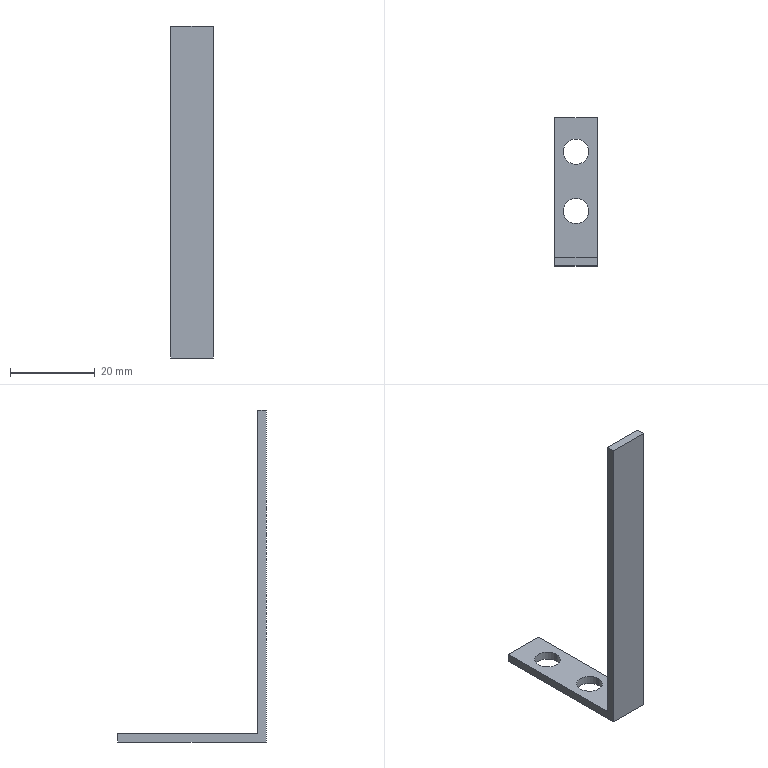Part | STEP file | 1_id1586_x_t | 1 solid | 12 faces | box 10 x 35 x 78.24 mm | volume 2112 mm3 | plane 8 | cylinder 4 | commonest cylinder face diameters 6 x4
STEP:
#1=CARTESIAN_POINT('',(0.,0.,0.));
#2=DIRECTION('',(0.,0.,1.));
#3=DIRECTION('',(1.,0.,0.));
#4=AXIS2_PLACEMENT_3D('',#1,#2,#3);
#5=CARTESIAN_POINT('',(897.895,192.425,-90.));
#6=VERTEX_POINT('',#5);
#7=CARTESIAN_POINT('',(897.895,192.425,-11.76));
#8=VERTEX_POINT('',#7);
#9=CARTESIAN_POINT('',(897.895,192.425,-90.));
#10=DIRECTION('',(0.,0.,1.));
#11=VECTOR('',#10,1.);
#12=LINE('',#9,#11);
#13=CARTESIAN_POINT('',(892.895,192.425,-50.88));
#14=DIRECTION('',(0.,1.,0.));
#15=DIRECTION('',(-1.,0.,0.));
#16=AXIS2_PLACEMENT_3D('',#13,#14,#15);
#17=PLANE('',#16);
#18=CARTESIAN_POINT('',(-5.,-39.12));
#19=DIRECTION('',(0.,1.));
#20=VECTOR('',#19,1.);
#21=LINE('',#18,#20);
#22=(GEOMETRIC_REPRESENTATION_CONTEXT(2)PARAMETRIC_REPRESENTATION_CONTEXT()REPRESENTATION_CONTEXT('',''));
#23=DEFINITIONAL_REPRESENTATION('',(#21),#22);
#24=PCURVE('',#17,#23);
#25=CARTESIAN_POINT('',(897.895,49.757,-105.374));
#26=DIRECTION('',(1.,0.,0.));
#27=DIRECTION('',(0.,-1.,0.));
#28=AXIS2_PLACEMENT_3D('',#25,#26,#27);
#29=PLANE('',#28);
#30=CARTESIAN_POINT('',(-142.668,-15.374));
#31=DIRECTION('',(0.,-1.));
#32=VECTOR('',#31,1.);
#33=LINE('',#30,#32);
#34=(GEOMETRIC_REPRESENTATION_CONTEXT(2)PARAMETRIC_REPRESENTATION_CONTEXT()REPRESENTATION_CONTEXT('',''));
#35=DEFINITIONAL_REPRESENTATION('',(#33),#34);
#36=PCURVE('',#29,#35);
#37=SURFACE_CURVE('',#12,(#24,#36),.PCURVE_S1.);
#38=EDGE_CURVE('',#6,#8,#37,.T.);
#39=ORIENTED_EDGE('',*,*,#38,.T.);
#40=CARTESIAN_POINT('',(887.895,192.425,-11.76));
#41=VERTEX_POINT('',#40);
#42=CARTESIAN_POINT('',(897.895,192.425,-11.76));
#43=DIRECTION('',(-1.,0.,0.));
#44=VECTOR('',#43,1.);
#45=LINE('',#42,#44);
#46=CARTESIAN_POINT('',(-5.,39.12));
#47=DIRECTION('',(1.,0.));
#48=VECTOR('',#47,1.);
#49=LINE('',#46,#48);
#50=(GEOMETRIC_REPRESENTATION_CONTEXT(2)PARAMETRIC_REPRESENTATION_CONTEXT()REPRESENTATION_CONTEXT('',''));
#51=DEFINITIONAL_REPRESENTATION('',(#49),#50);
#52=PCURVE('',#17,#51);
#53=CARTESIAN_POINT('',(902.895,192.425,-11.76));
#54=DIRECTION('',(0.,0.,-1.));
#55=DIRECTION('',(1.,0.,0.));
#56=AXIS2_PLACEMENT_3D('',#53,#54,#55);
#57=PLANE('',#56);
#58=CARTESIAN_POINT('',(-5.,0.));
#59=DIRECTION('',(-1.,0.));
#60=VECTOR('',#59,1.);
#61=LINE('',#58,#60);
#62=(GEOMETRIC_REPRESENTATION_CONTEXT(2)PARAMETRIC_REPRESENTATION_CONTEXT()REPRESENTATION_CONTEXT('',''));
#63=DEFINITIONAL_REPRESENTATION('',(#61),#62);
#64=PCURVE('',#57,#63);
#65=SURFACE_CURVE('',#45,(#52,#64),.PCURVE_S1.);
#66=EDGE_CURVE('',#8,#41,#65,.T.);
#67=ORIENTED_EDGE('',*,*,#66,.T.);
#68=CARTESIAN_POINT('',(887.895,192.425,-90.));
#69=VERTEX_POINT('',#68);
#70=CARTESIAN_POINT('',(887.895,192.425,-11.76));
#71=DIRECTION('',(0.,0.,-1.));
#72=VECTOR('',#71,1.);
#73=LINE('',#70,#72);
#74=CARTESIAN_POINT('',(5.,39.12));
#75=DIRECTION('',(0.,-1.));
#76=VECTOR('',#75,1.);
#77=LINE('',#74,#76);
#78=(GEOMETRIC_REPRESENTATION_CONTEXT(2)PARAMETRIC_REPRESENTATION_CONTEXT()REPRESENTATION_CONTEXT('',''));
#79=DEFINITIONAL_REPRESENTATION('',(#77),#78);
#80=PCURVE('',#17,#79);
#81=CARTESIAN_POINT('',(887.895,372.897,-105.638));
#82=DIRECTION('',(-1.,0.,0.));
#83=DIRECTION('',(0.,0.,-1.));
#84=AXIS2_PLACEMENT_3D('',#81,#82,#83);
#85=PLANE('',#84);
#86=CARTESIAN_POINT('',(-93.878,180.472));
#87=DIRECTION('',(1.,0.));
#88=VECTOR('',#87,1.);
#89=LINE('',#86,#88);
#90=(GEOMETRIC_REPRESENTATION_CONTEXT(2)PARAMETRIC_REPRESENTATION_CONTEXT()REPRESENTATION_CONTEXT('',''));
#91=DEFINITIONAL_REPRESENTATION('',(#89),#90);
#92=PCURVE('',#85,#91);
#93=SURFACE_CURVE('',#73,(#80,#92),.PCURVE_S1.);
#94=EDGE_CURVE('',#41,#69,#93,.T.);
#95=ORIENTED_EDGE('',*,*,#94,.T.);
#96=CARTESIAN_POINT('',(887.895,192.425,-90.));
#97=DIRECTION('',(1.,0.,0.));
#98=VECTOR('',#97,1.);
#99=LINE('',#96,#98);
#100=CARTESIAN_POINT('',(5.,-39.12));
#101=DIRECTION('',(-1.,0.));
#102=VECTOR('',#101,1.);
#103=LINE('',#100,#102);
#104=(GEOMETRIC_REPRESENTATION_CONTEXT(2)PARAMETRIC_REPRESENTATION_CONTEXT()REPRESENTATION_CONTEXT('',''));
#105=DEFINITIONAL_REPRESENTATION('',(#103),#104);
#106=PCURVE('',#17,#105);
#107=CARTESIAN_POINT('',(893.895,203.675,-90.));
#108=DIRECTION('',(0.,0.,-1.));
#109=DIRECTION('',(0.,1.,0.));
#110=AXIS2_PLACEMENT_3D('',#107,#108,#109);
#111=PLANE('',#110);
#112=CARTESIAN_POINT('',(-11.25,-6.));
#113=DIRECTION('',(0.,1.));
#114=VECTOR('',#113,1.);
#115=LINE('',#112,#114);
#116=(GEOMETRIC_REPRESENTATION_CONTEXT(2)PARAMETRIC_REPRESENTATION_CONTEXT()REPRESENTATION_CONTEXT('',''));
#117=DEFINITIONAL_REPRESENTATION('',(#115),#116);
#118=PCURVE('',#111,#117);
#119=SURFACE_CURVE('',#99,(#106,#118),.PCURVE_S1.);
#120=EDGE_CURVE('',#69,#6,#119,.T.);
#121=ORIENTED_EDGE('',*,*,#120,.T.);
#122=EDGE_LOOP('',(#39,#67,#95,#121));
#123=FACE_BOUND('',#122,.T.);
#124=ADVANCED_FACE('',(#123),#17,.F.);
#125=CARTESIAN_POINT('',(897.895,227.425,-90.));
#126=VERTEX_POINT('',#125);
#127=CARTESIAN_POINT('',(897.895,192.425,-90.));
#128=DIRECTION('',(0.,1.,0.));
#129=VECTOR('',#128,1.);
#130=LINE('',#127,#129);
#131=CARTESIAN_POINT('',(-11.25,4.));
#132=DIRECTION('',(1.,0.));
#133=VECTOR('',#132,1.);
#134=LINE('',#131,#133);
#135=(GEOMETRIC_REPRESENTATION_CONTEXT(2)PARAMETRIC_REPRESENTATION_CONTEXT()REPRESENTATION_CONTEXT('',''));
#136=DEFINITIONAL_REPRESENTATION('',(#134),#135);
#137=PCURVE('',#111,#136);
#138=CARTESIAN_POINT('',(-142.668,-15.374));
#139=DIRECTION('',(-1.,0.));
#140=VECTOR('',#139,1.);
#141=LINE('',#138,#140);
#142=(GEOMETRIC_REPRESENTATION_CONTEXT(2)PARAMETRIC_REPRESENTATION_CONTEXT()REPRESENTATION_CONTEXT('',''));
#143=DEFINITIONAL_REPRESENTATION('',(#141),#142);
#144=PCURVE('',#29,#143);
#145=SURFACE_CURVE('',#130,(#137,#144),.PCURVE_S1.);
#146=EDGE_CURVE('',#6,#126,#145,.T.);
#147=ORIENTED_EDGE('',*,*,#146,.F.);
#148=ORIENTED_EDGE('',*,*,#120,.F.);
#149=CARTESIAN_POINT('',(887.895,227.425,-90.));
#150=VERTEX_POINT('',#149);
#151=CARTESIAN_POINT('',(887.895,227.425,-90.));
#152=DIRECTION('',(0.,-1.,0.));
#153=VECTOR('',#152,1.);
#154=LINE('',#151,#153);
#155=CARTESIAN_POINT('',(23.75,-6.));
#156=DIRECTION('',(-1.,0.));
#157=VECTOR('',#156,1.);
#158=LINE('',#155,#157);
#159=(GEOMETRIC_REPRESENTATION_CONTEXT(2)PARAMETRIC_REPRESENTATION_CONTEXT()REPRESENTATION_CONTEXT('',''));
#160=DEFINITIONAL_REPRESENTATION('',(#158),#159);
#161=PCURVE('',#111,#160);
#162=CARTESIAN_POINT('',(-15.638,145.472));
#163=DIRECTION('',(0.,1.));
#164=VECTOR('',#163,1.);
#165=LINE('',#162,#164);
#166=(GEOMETRIC_REPRESENTATION_CONTEXT(2)PARAMETRIC_REPRESENTATION_CONTEXT()REPRESENTATION_CONTEXT('',''));
#167=DEFINITIONAL_REPRESENTATION('',(#165),#166);
#168=PCURVE('',#85,#167);
#169=SURFACE_CURVE('',#154,(#161,#168),.PCURVE_S1.);
#170=EDGE_CURVE('',#150,#69,#169,.T.);
#171=ORIENTED_EDGE('',*,*,#170,.F.);
#172=CARTESIAN_POINT('',(897.895,227.425,-90.));
#173=DIRECTION('',(-1.,0.,0.));
#174=VECTOR('',#173,1.);
#175=LINE('',#172,#174);
#176=CARTESIAN_POINT('',(23.75,4.));
#177=DIRECTION('',(0.,-1.));
#178=VECTOR('',#177,1.);
#179=LINE('',#176,#178);
#180=(GEOMETRIC_REPRESENTATION_CONTEXT(2)PARAMETRIC_REPRESENTATION_CONTEXT()REPRESENTATION_CONTEXT('',''));
#181=DEFINITIONAL_REPRESENTATION('',(#179),#180);
#182=PCURVE('',#111,#181);
#183=CARTESIAN_POINT('',(893.895,227.425,-90.));
#184=DIRECTION('',(0.,1.,0.));
#185=DIRECTION('',(-1.,0.,0.));
#186=AXIS2_PLACEMENT_3D('',#183,#184,#185);
#187=PLANE('',#186);
#188=CARTESIAN_POINT('',(-4.,0.));
#189=DIRECTION('',(1.,0.));
#190=VECTOR('',#189,1.);
#191=LINE('',#188,#190);
#192=(GEOMETRIC_REPRESENTATION_CONTEXT(2)PARAMETRIC_REPRESENTATION_CONTEXT()REPRESENTATION_CONTEXT('',''));
#193=DEFINITIONAL_REPRESENTATION('',(#191),#192);
#194=PCURVE('',#187,#193);
#195=SURFACE_CURVE('',#175,(#182,#194),.PCURVE_S1.);
#196=EDGE_CURVE('',#126,#150,#195,.T.);
#197=ORIENTED_EDGE('',*,*,#196,.F.);
#198=EDGE_LOOP('',(#147,#148,#171,#197));
#199=FACE_BOUND('',#198,.T.);
#200=CARTESIAN_POINT('',(895.895,219.425,-90.));
#201=VERTEX_POINT('',#200);
#202=CARTESIAN_POINT('',(889.895,219.425,-90.));
#203=VERTEX_POINT('',#202);
#204=CARTESIAN_POINT('',(892.895,219.425,-90.));
#205=DIRECTION('',(0.,0.,1.));
#206=DIRECTION('',(1.,0.,0.));
#207=AXIS2_PLACEMENT_3D('',#204,#205,#206);
#208=CIRCLE('',#207,3.);
#209=CARTESIAN_POINT('',(15.75,2.));
#210=CARTESIAN_POINT('',(20.946,2.));
#211=CARTESIAN_POINT('',(18.348,-2.5));
#212=CARTESIAN_POINT('',(15.75,-7.));
#213=CARTESIAN_POINT('',(13.152,-2.5));
#214=CARTESIAN_POINT('',(10.554,2.));
#215=CARTESIAN_POINT('',(15.75,2.));
#216=(BOUNDED_CURVE()B_SPLINE_CURVE(2,(#209,#210,#211,#212,#213,#214,#215),.UNSPECIFIED.,.T.,.F.)B_SPLINE_CURVE_WITH_KNOTS((1,2,2,2,2,1),(-2.094,0.,2.094,4.189,6.283,8.378),.UNSPECIFIED.)CURVE()GEOMETRIC_REPRESENTATION_ITEM()RATIONAL_B_SPLINE_CURVE((1.,0.5,1.,0.5,1.,0.5,1.))REPRESENTATION_ITEM(''));
#217=(GEOMETRIC_REPRESENTATION_CONTEXT(2)PARAMETRIC_REPRESENTATION_CONTEXT()REPRESENTATION_CONTEXT('',''));
#218=DEFINITIONAL_REPRESENTATION('',(#216),#217);
#219=PCURVE('',#111,#218);
#220=CARTESIAN_POINT('',(892.895,219.425,-94.25));
#221=DIRECTION('',(0.,0.,-1.));
#222=DIRECTION('',(-1.,0.,0.));
#223=AXIS2_PLACEMENT_3D('',#220,#221,#222);
#224=CYLINDRICAL_SURFACE('',#223,3.);
#225=CARTESIAN_POINT('',(3.142,-4.25));
#226=DIRECTION('',(-1.,0.));
#227=VECTOR('',#226,1.);
#228=LINE('',#225,#227);
#229=(GEOMETRIC_REPRESENTATION_CONTEXT(2)PARAMETRIC_REPRESENTATION_CONTEXT()REPRESENTATION_CONTEXT('',''));
#230=DEFINITIONAL_REPRESENTATION('',(#228),#229);
#231=PCURVE('',#224,#230);
#232=SURFACE_CURVE('',#208,(#219,#231),.PCURVE_S1.);
#233=EDGE_CURVE('',#201,#203,#232,.T.);
#234=ORIENTED_EDGE('',*,*,#233,.T.);
#235=CARTESIAN_POINT('',(892.895,219.425,-90.));
#236=DIRECTION('',(0.,0.,1.));
#237=DIRECTION('',(-1.,0.,0.));
#238=AXIS2_PLACEMENT_3D('',#235,#236,#237);
#239=CIRCLE('',#238,3.);
#240=CARTESIAN_POINT('',(15.75,-4.));
#241=CARTESIAN_POINT('',(10.554,-4.));
#242=CARTESIAN_POINT('',(13.152,0.5));
#243=CARTESIAN_POINT('',(15.75,5.));
#244=CARTESIAN_POINT('',(18.348,0.5));
#245=CARTESIAN_POINT('',(20.946,-4.));
#246=CARTESIAN_POINT('',(15.75,-4.));
#247=(BOUNDED_CURVE()B_SPLINE_CURVE(2,(#240,#241,#242,#243,#244,#245,#246),.UNSPECIFIED.,.T.,.F.)B_SPLINE_CURVE_WITH_KNOTS((1,2,2,2,2,1),(-2.094,0.,2.094,4.189,6.283,8.378),.UNSPECIFIED.)CURVE()GEOMETRIC_REPRESENTATION_ITEM()RATIONAL_B_SPLINE_CURVE((1.,0.5,1.,0.5,1.,0.5,1.))REPRESENTATION_ITEM(''));
#248=(GEOMETRIC_REPRESENTATION_CONTEXT(2)PARAMETRIC_REPRESENTATION_CONTEXT()REPRESENTATION_CONTEXT('',''));
#249=DEFINITIONAL_REPRESENTATION('',(#247),#248);
#250=PCURVE('',#111,#249);
#251=CARTESIAN_POINT('',(892.895,219.425,-94.25));
#252=DIRECTION('',(0.,0.,-1.));
#253=DIRECTION('',(-1.,0.,0.));
#254=AXIS2_PLACEMENT_3D('',#251,#252,#253);
#255=CYLINDRICAL_SURFACE('',#254,3.);
#256=CARTESIAN_POINT('',(6.283,-4.25));
#257=DIRECTION('',(-1.,0.));
#258=VECTOR('',#257,1.);
#259=LINE('',#256,#258);
#260=(GEOMETRIC_REPRESENTATION_CONTEXT(2)PARAMETRIC_REPRESENTATION_CONTEXT()REPRESENTATION_CONTEXT('',''));
#261=DEFINITIONAL_REPRESENTATION('',(#259),#260);
#262=PCURVE('',#255,#261);
#263=SURFACE_CURVE('',#239,(#250,#262),.PCURVE_S1.);
#264=EDGE_CURVE('',#203,#201,#263,.T.);
#265=ORIENTED_EDGE('',*,*,#264,.T.);
#266=EDGE_LOOP('',(#234,#265));
#267=FACE_BOUND('',#266,.T.);
#268=CARTESIAN_POINT('',(895.895,205.425,-90.));
#269=VERTEX_POINT('',#268);
#270=CARTESIAN_POINT('',(889.895,205.425,-90.));
#271=VERTEX_POINT('',#270);
#272=CARTESIAN_POINT('',(892.895,205.425,-90.));
#273=DIRECTION('',(0.,0.,1.));
#274=DIRECTION('',(1.,0.,0.));
#275=AXIS2_PLACEMENT_3D('',#272,#273,#274);
#276=CIRCLE('',#275,3.);
#277=CARTESIAN_POINT('',(1.75,2.));
#278=CARTESIAN_POINT('',(6.946,2.));
#279=CARTESIAN_POINT('',(4.348,-2.5));
#280=CARTESIAN_POINT('',(1.75,-7.));
#281=CARTESIAN_POINT('',(-0.8481,-2.5));
#282=CARTESIAN_POINT('',(-3.446,2.));
#283=CARTESIAN_POINT('',(1.75,2.));
#284=(BOUNDED_CURVE()B_SPLINE_CURVE(2,(#277,#278,#279,#280,#281,#282,#283),.UNSPECIFIED.,.T.,.F.)B_SPLINE_CURVE_WITH_KNOTS((1,2,2,2,2,1),(-2.094,0.,2.094,4.189,6.283,8.378),.UNSPECIFIED.)CURVE()GEOMETRIC_REPRESENTATION_ITEM()RATIONAL_B_SPLINE_CURVE((1.,0.5,1.,0.5,1.,0.5,1.))REPRESENTATION_ITEM(''));
#285=(GEOMETRIC_REPRESENTATION_CONTEXT(2)PARAMETRIC_REPRESENTATION_CONTEXT()REPRESENTATION_CONTEXT('',''));
#286=DEFINITIONAL_REPRESENTATION('',(#284),#285);
#287=PCURVE('',#111,#286);
#288=CARTESIAN_POINT('',(892.895,205.425,-94.25));
#289=DIRECTION('',(0.,0.,-1.));
#290=DIRECTION('',(1.,0.,0.));
#291=AXIS2_PLACEMENT_3D('',#288,#289,#290);
#292=CYLINDRICAL_SURFACE('',#291,3.);
#293=CARTESIAN_POINT('',(6.283,-4.25));
#294=DIRECTION('',(-1.,0.));
#295=VECTOR('',#294,1.);
#296=LINE('',#293,#295);
#297=(GEOMETRIC_REPRESENTATION_CONTEXT(2)PARAMETRIC_REPRESENTATION_CONTEXT()REPRESENTATION_CONTEXT('',''));
#298=DEFINITIONAL_REPRESENTATION('',(#296),#297);
#299=PCURVE('',#292,#298);
#300=SURFACE_CURVE('',#276,(#287,#299),.PCURVE_S1.);
#301=EDGE_CURVE('',#269,#271,#300,.T.);
#302=ORIENTED_EDGE('',*,*,#301,.T.);
#303=CARTESIAN_POINT('',(892.895,205.425,-90.));
#304=DIRECTION('',(0.,0.,1.));
#305=DIRECTION('',(-1.,0.,0.));
#306=AXIS2_PLACEMENT_3D('',#303,#304,#305);
#307=CIRCLE('',#306,3.);
#308=CARTESIAN_POINT('',(1.75,-4.));
#309=CARTESIAN_POINT('',(-3.446,-4.));
#310=CARTESIAN_POINT('',(-0.8481,0.5));
#311=CARTESIAN_POINT('',(1.75,5.));
#312=CARTESIAN_POINT('',(4.348,0.5));
#313=CARTESIAN_POINT('',(6.946,-4.));
#314=CARTESIAN_POINT('',(1.75,-4.));
#315=(BOUNDED_CURVE()B_SPLINE_CURVE(2,(#308,#309,#310,#311,#312,#313,#314),.UNSPECIFIED.,.T.,.F.)B_SPLINE_CURVE_WITH_KNOTS((1,2,2,2,2,1),(-2.094,0.,2.094,4.189,6.283,8.378),.UNSPECIFIED.)CURVE()GEOMETRIC_REPRESENTATION_ITEM()RATIONAL_B_SPLINE_CURVE((1.,0.5,1.,0.5,1.,0.5,1.))REPRESENTATION_ITEM(''));
#316=(GEOMETRIC_REPRESENTATION_CONTEXT(2)PARAMETRIC_REPRESENTATION_CONTEXT()REPRESENTATION_CONTEXT('',''));
#317=DEFINITIONAL_REPRESENTATION('',(#315),#316);
#318=PCURVE('',#111,#317);
#319=CARTESIAN_POINT('',(892.895,205.425,-94.25));
#320=DIRECTION('',(0.,0.,-1.));
#321=DIRECTION('',(1.,0.,0.));
#322=AXIS2_PLACEMENT_3D('',#319,#320,#321);
#323=CYLINDRICAL_SURFACE('',#322,3.);
#324=CARTESIAN_POINT('',(3.142,-4.25));
#325=DIRECTION('',(-1.,0.));
#326=VECTOR('',#325,1.);
#327=LINE('',#324,#326);
#328=(GEOMETRIC_REPRESENTATION_CONTEXT(2)PARAMETRIC_REPRESENTATION_CONTEXT()REPRESENTATION_CONTEXT('',''));
#329=DEFINITIONAL_REPRESENTATION('',(#327),#328);
#330=PCURVE('',#323,#329);
#331=SURFACE_CURVE('',#307,(#318,#330),.PCURVE_S1.);
#332=EDGE_CURVE('',#271,#269,#331,.T.);
#333=ORIENTED_EDGE('',*,*,#332,.T.);
#334=EDGE_LOOP('',(#302,#333));
#335=FACE_BOUND('',#334,.T.);
#336=ADVANCED_FACE('',(#199,#267,#335),#111,.T.);
#337=ORIENTED_EDGE('',*,*,#196,.T.);
#338=CARTESIAN_POINT('',(887.895,227.425,-88.));
#339=VERTEX_POINT('',#338);
#340=CARTESIAN_POINT('',(887.895,227.425,-90.));
#341=DIRECTION('',(0.,0.,1.));
#342=VECTOR('',#341,1.);
#343=LINE('',#340,#342);
#344=CARTESIAN_POINT('',(6.,0.));
#345=DIRECTION('',(0.,1.));
#346=VECTOR('',#345,1.);
#347=LINE('',#344,#346);
#348=(GEOMETRIC_REPRESENTATION_CONTEXT(2)PARAMETRIC_REPRESENTATION_CONTEXT()REPRESENTATION_CONTEXT('',''));
#349=DEFINITIONAL_REPRESENTATION('',(#347),#348);
#350=PCURVE('',#187,#349);
#351=CARTESIAN_POINT('',(-15.638,145.472));
#352=DIRECTION('',(-1.,0.));
#353=VECTOR('',#352,1.);
#354=LINE('',#351,#353);
#355=(GEOMETRIC_REPRESENTATION_CONTEXT(2)PARAMETRIC_REPRESENTATION_CONTEXT()REPRESENTATION_CONTEXT('',''));
#356=DEFINITIONAL_REPRESENTATION('',(#354),#355);
#357=PCURVE('',#85,#356);
#358=SURFACE_CURVE('',#343,(#350,#357),.PCURVE_S1.);
#359=EDGE_CURVE('',#150,#339,#358,.T.);
#360=ORIENTED_EDGE('',*,*,#359,.T.);
#361=CARTESIAN_POINT('',(897.895,227.425,-88.));
#362=VERTEX_POINT('',#361);
#363=CARTESIAN_POINT('',(897.895,227.425,-88.));
#364=DIRECTION('',(-1.,0.,0.));
#365=VECTOR('',#364,1.);
#366=LINE('',#363,#365);
#367=CARTESIAN_POINT('',(-4.,2.));
#368=DIRECTION('',(1.,0.));
#369=VECTOR('',#368,1.);
#370=LINE('',#367,#369);
#371=(GEOMETRIC_REPRESENTATION_CONTEXT(2)PARAMETRIC_REPRESENTATION_CONTEXT()REPRESENTATION_CONTEXT('',''));
#372=DEFINITIONAL_REPRESENTATION('',(#370),#371);
#373=PCURVE('',#187,#372);
#374=CARTESIAN_POINT('',(893.895,203.675,-88.));
#375=DIRECTION('',(0.,0.,-1.));
#376=DIRECTION('',(0.,1.,0.));
#377=AXIS2_PLACEMENT_3D('',#374,#375,#376);
#378=PLANE('',#377);
#379=CARTESIAN_POINT('',(23.75,4.));
#380=DIRECTION('',(0.,-1.));
#381=VECTOR('',#380,1.);
#382=LINE('',#379,#381);
#383=(GEOMETRIC_REPRESENTATION_CONTEXT(2)PARAMETRIC_REPRESENTATION_CONTEXT()REPRESENTATION_CONTEXT('',''));
#384=DEFINITIONAL_REPRESENTATION('',(#382),#383);
#385=PCURVE('',#378,#384);
#386=SURFACE_CURVE('',#366,(#373,#385),.PCURVE_S1.);
#387=EDGE_CURVE('',#362,#339,#386,.T.);
#388=ORIENTED_EDGE('',*,*,#387,.F.);
#389=CARTESIAN_POINT('',(897.895,227.425,-88.));
#390=DIRECTION('',(0.,0.,-1.));
#391=VECTOR('',#390,1.);
#392=LINE('',#389,#391);
#393=CARTESIAN_POINT('',(-4.,2.));
#394=DIRECTION('',(0.,-1.));
#395=VECTOR('',#394,1.);
#396=LINE('',#393,#395);
#397=(GEOMETRIC_REPRESENTATION_CONTEXT(2)PARAMETRIC_REPRESENTATION_CONTEXT()REPRESENTATION_CONTEXT('',''));
#398=DEFINITIONAL_REPRESENTATION('',(#396),#397);
#399=PCURVE('',#187,#398);
#400=CARTESIAN_POINT('',(-177.668,-17.374));
#401=DIRECTION('',(0.,1.));
#402=VECTOR('',#401,1.);
#403=LINE('',#400,#402);
#404=(GEOMETRIC_REPRESENTATION_CONTEXT(2)PARAMETRIC_REPRESENTATION_CONTEXT()REPRESENTATION_CONTEXT('',''));
#405=DEFINITIONAL_REPRESENTATION('',(#403),#404);
#406=PCURVE('',#29,#405);
#407=SURFACE_CURVE('',#392,(#399,#406),.PCURVE_S1.);
#408=EDGE_CURVE('',#362,#126,#407,.T.);
#409=ORIENTED_EDGE('',*,*,#408,.T.);
#410=EDGE_LOOP('',(#337,#360,#388,#409));
#411=FACE_BOUND('',#410,.T.);
#412=ADVANCED_FACE('',(#411),#187,.T.);
#413=CARTESIAN_POINT('',(897.895,194.425,-88.));
#414=VERTEX_POINT('',#413);
#415=CARTESIAN_POINT('',(897.895,194.425,-88.));
#416=DIRECTION('',(0.,1.,0.));
#417=VECTOR('',#416,1.);
#418=LINE('',#415,#417);
#419=CARTESIAN_POINT('',(-144.668,-17.374));
#420=DIRECTION('',(-1.,0.));
#421=VECTOR('',#420,1.);
#422=LINE('',#419,#421);
#423=(GEOMETRIC_REPRESENTATION_CONTEXT(2)PARAMETRIC_REPRESENTATION_CONTEXT()REPRESENTATION_CONTEXT('',''));
#424=DEFINITIONAL_REPRESENTATION('',(#422),#423);
#425=PCURVE('',#29,#424);
#426=CARTESIAN_POINT('',(-9.25,4.));
#427=DIRECTION('',(1.,0.));
#428=VECTOR('',#427,1.);
#429=LINE('',#426,#428);
#430=(GEOMETRIC_REPRESENTATION_CONTEXT(2)PARAMETRIC_REPRESENTATION_CONTEXT()REPRESENTATION_CONTEXT('',''));
#431=DEFINITIONAL_REPRESENTATION('',(#429),#430);
#432=PCURVE('',#378,#431);
#433=SURFACE_CURVE('',#418,(#425,#432),.PCURVE_S1.);
#434=EDGE_CURVE('',#414,#362,#433,.T.);
#435=ORIENTED_EDGE('',*,*,#434,.F.);
#436=CARTESIAN_POINT('',(897.895,194.425,-11.76));
#437=VERTEX_POINT('',#436);
#438=CARTESIAN_POINT('',(897.895,194.425,-11.76));
#439=DIRECTION('',(0.,0.,-1.));
#440=VECTOR('',#439,1.);
#441=LINE('',#438,#440);
#442=CARTESIAN_POINT('',(-144.668,-93.614));
#443=DIRECTION('',(0.,1.));
#444=VECTOR('',#443,1.);
#445=LINE('',#442,#444);
#446=(GEOMETRIC_REPRESENTATION_CONTEXT(2)PARAMETRIC_REPRESENTATION_CONTEXT()REPRESENTATION_CONTEXT('',''));
#447=DEFINITIONAL_REPRESENTATION('',(#445),#446);
#448=PCURVE('',#29,#447);
#449=CARTESIAN_POINT('',(892.895,194.425,-49.88));
#450=DIRECTION('',(0.,1.,0.));
#451=DIRECTION('',(1.,0.,0.));
#452=AXIS2_PLACEMENT_3D('',#449,#450,#451);
#453=PLANE('',#452);
#454=CARTESIAN_POINT('',(5.,-38.12));
#455=DIRECTION('',(0.,1.));
#456=VECTOR('',#455,1.);
#457=LINE('',#454,#456);
#458=(GEOMETRIC_REPRESENTATION_CONTEXT(2)PARAMETRIC_REPRESENTATION_CONTEXT()REPRESENTATION_CONTEXT('',''));
#459=DEFINITIONAL_REPRESENTATION('',(#457),#458);
#460=PCURVE('',#453,#459);
#461=SURFACE_CURVE('',#441,(#448,#460),.PCURVE_S1.);
#462=EDGE_CURVE('',#437,#414,#461,.T.);
#463=ORIENTED_EDGE('',*,*,#462,.F.);
#464=CARTESIAN_POINT('',(897.895,192.425,-11.76));
#465=DIRECTION('',(0.,1.,0.));
#466=VECTOR('',#465,1.);
#467=LINE('',#464,#466);
#468=CARTESIAN_POINT('',(-142.668,-93.614));
#469=DIRECTION('',(-1.,0.));
#470=VECTOR('',#469,1.);
#471=LINE('',#468,#470);
#472=(GEOMETRIC_REPRESENTATION_CONTEXT(2)PARAMETRIC_REPRESENTATION_CONTEXT()REPRESENTATION_CONTEXT('',''));
#473=DEFINITIONAL_REPRESENTATION('',(#471),#472);
#474=PCURVE('',#29,#473);
#475=CARTESIAN_POINT('',(-5.,0.));
#476=DIRECTION('',(0.,-1.));
#477=VECTOR('',#476,1.);
#478=LINE('',#475,#477);
#479=(GEOMETRIC_REPRESENTATION_CONTEXT(2)PARAMETRIC_REPRESENTATION_CONTEXT()REPRESENTATION_CONTEXT('',''));
#480=DEFINITIONAL_REPRESENTATION('',(#478),#479);
#481=PCURVE('',#57,#480);
#482=SURFACE_CURVE('',#467,(#474,#481),.PCURVE_S1.);
#483=EDGE_CURVE('',#8,#437,#482,.T.);
#484=ORIENTED_EDGE('',*,*,#483,.F.);
#485=ORIENTED_EDGE('',*,*,#38,.F.);
#486=ORIENTED_EDGE('',*,*,#146,.T.);
#487=ORIENTED_EDGE('',*,*,#408,.F.);
#488=EDGE_LOOP('',(#435,#463,#484,#485,#486,#487));
#489=FACE_BOUND('',#488,.T.);
#490=ADVANCED_FACE('',(#489),#29,.T.);
#491=CARTESIAN_POINT('',(887.895,194.425,-11.76));
#492=VERTEX_POINT('',#491);
#493=CARTESIAN_POINT('',(887.895,194.425,-11.76));
#494=DIRECTION('',(1.,0.,0.));
#495=VECTOR('',#494,1.);
#496=LINE('',#493,#495);
#497=CARTESIAN_POINT('',(-15.,-2.));
#498=DIRECTION('',(1.,0.));
#499=VECTOR('',#498,1.);
#500=LINE('',#497,#499);
#501=(GEOMETRIC_REPRESENTATION_CONTEXT(2)PARAMETRIC_REPRESENTATION_CONTEXT()REPRESENTATION_CONTEXT('',''));
#502=DEFINITIONAL_REPRESENTATION('',(#500),#501);
#503=PCURVE('',#57,#502);
#504=CARTESIAN_POINT('',(-5.,-38.12));
#505=DIRECTION('',(1.,0.));
#506=VECTOR('',#505,1.);
#507=LINE('',#504,#506);
#508=(GEOMETRIC_REPRESENTATION_CONTEXT(2)PARAMETRIC_REPRESENTATION_CONTEXT()REPRESENTATION_CONTEXT('',''));
#509=DEFINITIONAL_REPRESENTATION('',(#507),#508);
#510=PCURVE('',#453,#509);
#511=SURFACE_CURVE('',#496,(#503,#510),.PCURVE_S1.);
#512=EDGE_CURVE('',#492,#437,#511,.T.);
#513=ORIENTED_EDGE('',*,*,#512,.F.);
#514=CARTESIAN_POINT('',(887.895,194.425,-11.76));
#515=DIRECTION('',(0.,-1.,0.));
#516=VECTOR('',#515,1.);
#517=LINE('',#514,#516);
#518=CARTESIAN_POINT('',(-15.,-2.));
#519=DIRECTION('',(0.,1.));
#520=VECTOR('',#519,1.);
#521=LINE('',#518,#520);
#522=(GEOMETRIC_REPRESENTATION_CONTEXT(2)PARAMETRIC_REPRESENTATION_CONTEXT()REPRESENTATION_CONTEXT('',''));
#523=DEFINITIONAL_REPRESENTATION('',(#521),#522);
#524=PCURVE('',#57,#523);
#525=CARTESIAN_POINT('',(-93.878,178.472));
#526=DIRECTION('',(0.,1.));
#527=VECTOR('',#526,1.);
#528=LINE('',#525,#527);
#529=(GEOMETRIC_REPRESENTATION_CONTEXT(2)PARAMETRIC_REPRESENTATION_CONTEXT()REPRESENTATION_CONTEXT('',''));
#530=DEFINITIONAL_REPRESENTATION('',(#528),#529);
#531=PCURVE('',#85,#530);
#532=SURFACE_CURVE('',#517,(#524,#531),.PCURVE_S1.);
#533=EDGE_CURVE('',#492,#41,#532,.T.);
#534=ORIENTED_EDGE('',*,*,#533,.T.);
#535=ORIENTED_EDGE('',*,*,#66,.F.);
#536=ORIENTED_EDGE('',*,*,#483,.T.);
#537=EDGE_LOOP('',(#513,#534,#535,#536));
#538=FACE_BOUND('',#537,.T.);
#539=ADVANCED_FACE('',(#538),#57,.F.);
#540=CARTESIAN_POINT('',(887.895,194.425,-88.));
#541=VERTEX_POINT('',#540);
#542=CARTESIAN_POINT('',(887.895,227.425,-88.));
#543=DIRECTION('',(0.,-1.,0.));
#544=VECTOR('',#543,1.);
#545=LINE('',#542,#544);
#546=CARTESIAN_POINT('',(-17.638,145.472));
#547=DIRECTION('',(0.,1.));
#548=VECTOR('',#547,1.);
#549=LINE('',#546,#548);
#550=(GEOMETRIC_REPRESENTATION_CONTEXT(2)PARAMETRIC_REPRESENTATION_CONTEXT()REPRESENTATION_CONTEXT('',''));
#551=DEFINITIONAL_REPRESENTATION('',(#549),#550);
#552=PCURVE('',#85,#551);
#553=CARTESIAN_POINT('',(23.75,-6.));
#554=DIRECTION('',(-1.,0.));
#555=VECTOR('',#554,1.);
#556=LINE('',#553,#555);
#557=(GEOMETRIC_REPRESENTATION_CONTEXT(2)PARAMETRIC_REPRESENTATION_CONTEXT()REPRESENTATION_CONTEXT('',''));
#558=DEFINITIONAL_REPRESENTATION('',(#556),#557);
#559=PCURVE('',#378,#558);
#560=SURFACE_CURVE('',#545,(#552,#559),.PCURVE_S1.);
#561=EDGE_CURVE('',#339,#541,#560,.T.);
#562=ORIENTED_EDGE('',*,*,#561,.F.);
#563=ORIENTED_EDGE('',*,*,#359,.F.);
#564=ORIENTED_EDGE('',*,*,#170,.T.);
#565=ORIENTED_EDGE('',*,*,#94,.F.);
#566=ORIENTED_EDGE('',*,*,#533,.F.);
#567=CARTESIAN_POINT('',(887.895,194.425,-88.));
#568=DIRECTION('',(0.,0.,1.));
#569=VECTOR('',#568,1.);
#570=LINE('',#567,#569);
#571=CARTESIAN_POINT('',(-17.638,178.472));
#572=DIRECTION('',(-1.,0.));
#573=VECTOR('',#572,1.);
#574=LINE('',#571,#573);
#575=(GEOMETRIC_REPRESENTATION_CONTEXT(2)PARAMETRIC_REPRESENTATION_CONTEXT()REPRESENTATION_CONTEXT('',''));
#576=DEFINITIONAL_REPRESENTATION('',(#574),#575);
#577=PCURVE('',#85,#576);
#578=CARTESIAN_POINT('',(-5.,38.12));
#579=DIRECTION('',(0.,-1.));
#580=VECTOR('',#579,1.);
#581=LINE('',#578,#580);
#582=(GEOMETRIC_REPRESENTATION_CONTEXT(2)PARAMETRIC_REPRESENTATION_CONTEXT()REPRESENTATION_CONTEXT('',''));
#583=DEFINITIONAL_REPRESENTATION('',(#581),#582);
#584=PCURVE('',#453,#583);
#585=SURFACE_CURVE('',#570,(#577,#584),.PCURVE_S1.);
#586=EDGE_CURVE('',#541,#492,#585,.T.);
#587=ORIENTED_EDGE('',*,*,#586,.F.);
#588=EDGE_LOOP('',(#562,#563,#564,#565,#566,#587));
#589=FACE_BOUND('',#588,.T.);
#590=ADVANCED_FACE('',(#589),#85,.T.);
#591=CARTESIAN_POINT('',(897.895,194.425,-88.));
#592=DIRECTION('',(-1.,0.,0.));
#593=VECTOR('',#592,1.);
#594=LINE('',#591,#593);
#595=CARTESIAN_POINT('',(5.,38.12));
#596=DIRECTION('',(-1.,0.));
#597=VECTOR('',#596,1.);
#598=LINE('',#595,#597);
#599=(GEOMETRIC_REPRESENTATION_CONTEXT(2)PARAMETRIC_REPRESENTATION_CONTEXT()REPRESENTATION_CONTEXT('',''));
#600=DEFINITIONAL_REPRESENTATION('',(#598),#599);
#601=PCURVE('',#453,#600);
#602=CARTESIAN_POINT('',(-9.25,4.));
#603=DIRECTION('',(0.,-1.));
#604=VECTOR('',#603,1.);
#605=LINE('',#602,#604);
#606=(GEOMETRIC_REPRESENTATION_CONTEXT(2)PARAMETRIC_REPRESENTATION_CONTEXT()REPRESENTATION_CONTEXT('',''));
#607=DEFINITIONAL_REPRESENTATION('',(#605),#606);
#608=PCURVE('',#378,#607);
#609=SURFACE_CURVE('',#594,(#601,#608),.PCURVE_S1.);
#610=EDGE_CURVE('',#414,#541,#609,.T.);
#611=ORIENTED_EDGE('',*,*,#610,.T.);
#612=ORIENTED_EDGE('',*,*,#586,.T.);
#613=ORIENTED_EDGE('',*,*,#512,.T.);
#614=ORIENTED_EDGE('',*,*,#462,.T.);
#615=EDGE_LOOP('',(#611,#612,#613,#614));
#616=FACE_BOUND('',#615,.T.);
#617=ADVANCED_FACE('',(#616),#453,.T.);
#618=ORIENTED_EDGE('',*,*,#387,.T.);
#619=ORIENTED_EDGE('',*,*,#561,.T.);
#620=ORIENTED_EDGE('',*,*,#610,.F.);
#621=ORIENTED_EDGE('',*,*,#434,.T.);
#622=EDGE_LOOP('',(#618,#619,#620,#621));
#623=FACE_BOUND('',#622,.T.);
#624=CARTESIAN_POINT('',(889.895,219.425,-88.));
#625=VERTEX_POINT('',#624);
#626=CARTESIAN_POINT('',(895.895,219.425,-88.));
#627=VERTEX_POINT('',#626);
#628=CARTESIAN_POINT('',(892.895,219.425,-88.));
#629=DIRECTION('',(0.,0.,-1.));
#630=DIRECTION('',(-1.,0.,0.));
#631=AXIS2_PLACEMENT_3D('',#628,#629,#630);
#632=CIRCLE('',#631,3.);
#633=CARTESIAN_POINT('',(15.75,-1.));
#634=DIRECTION('',(0.,-1.));
#635=AXIS2_PLACEMENT_2D('',#633,#634);
#636=CIRCLE('',#635,3.);
#637=(GEOMETRIC_REPRESENTATION_CONTEXT(2)PARAMETRIC_REPRESENTATION_CONTEXT()REPRESENTATION_CONTEXT('',''));
#638=DEFINITIONAL_REPRESENTATION('',(#636),#637);
#639=PCURVE('',#378,#638);
#640=CARTESIAN_POINT('',(0.,-6.25));
#641=DIRECTION('',(1.,0.));
#642=VECTOR('',#641,1.);
#643=LINE('',#640,#642);
#644=(GEOMETRIC_REPRESENTATION_CONTEXT(2)PARAMETRIC_REPRESENTATION_CONTEXT()REPRESENTATION_CONTEXT('',''));
#645=DEFINITIONAL_REPRESENTATION('',(#643),#644);
#646=PCURVE('',#224,#645);
#647=SURFACE_CURVE('',#632,(#639,#646),.PCURVE_S1.);
#648=EDGE_CURVE('',#625,#627,#647,.T.);
#649=ORIENTED_EDGE('',*,*,#648,.T.);
#650=CARTESIAN_POINT('',(892.895,219.425,-88.));
#651=DIRECTION('',(0.,0.,-1.));
#652=DIRECTION('',(1.,0.,0.));
#653=AXIS2_PLACEMENT_3D('',#650,#651,#652);
#654=CIRCLE('',#653,3.);
#655=CARTESIAN_POINT('',(15.75,-1.));
#656=DIRECTION('',(0.,1.));
#657=AXIS2_PLACEMENT_2D('',#655,#656);
#658=CIRCLE('',#657,3.);
#659=(GEOMETRIC_REPRESENTATION_CONTEXT(2)PARAMETRIC_REPRESENTATION_CONTEXT()REPRESENTATION_CONTEXT('',''));
#660=DEFINITIONAL_REPRESENTATION('',(#658),#659);
#661=PCURVE('',#378,#660);
#662=CARTESIAN_POINT('',(3.142,-6.25));
#663=DIRECTION('',(1.,0.));
#664=VECTOR('',#663,1.);
#665=LINE('',#662,#664);
#666=(GEOMETRIC_REPRESENTATION_CONTEXT(2)PARAMETRIC_REPRESENTATION_CONTEXT()REPRESENTATION_CONTEXT('',''));
#667=DEFINITIONAL_REPRESENTATION('',(#665),#666);
#668=PCURVE('',#255,#667);
#669=SURFACE_CURVE('',#654,(#661,#668),.PCURVE_S1.);
#670=EDGE_CURVE('',#627,#625,#669,.T.);
#671=ORIENTED_EDGE('',*,*,#670,.T.);
#672=EDGE_LOOP('',(#649,#671));
#673=FACE_BOUND('',#672,.T.);
#674=CARTESIAN_POINT('',(895.895,205.425,-88.));
#675=VERTEX_POINT('',#674);
#676=CARTESIAN_POINT('',(889.895,205.425,-88.));
#677=VERTEX_POINT('',#676);
#678=CARTESIAN_POINT('',(892.895,205.425,-88.));
#679=DIRECTION('',(0.,0.,-1.));
#680=DIRECTION('',(1.,0.,0.));
#681=AXIS2_PLACEMENT_3D('',#678,#679,#680);
#682=CIRCLE('',#681,3.);
#683=CARTESIAN_POINT('',(1.75,-1.));
#684=DIRECTION('',(0.,1.));
#685=AXIS2_PLACEMENT_2D('',#683,#684);
#686=CIRCLE('',#685,3.);
#687=(GEOMETRIC_REPRESENTATION_CONTEXT(2)PARAMETRIC_REPRESENTATION_CONTEXT()REPRESENTATION_CONTEXT('',''));
#688=DEFINITIONAL_REPRESENTATION('',(#686),#687);
#689=PCURVE('',#378,#688);
#690=CARTESIAN_POINT('',(0.,-6.25));
#691=DIRECTION('',(1.,0.));
#692=VECTOR('',#691,1.);
#693=LINE('',#690,#692);
#694=(GEOMETRIC_REPRESENTATION_CONTEXT(2)PARAMETRIC_REPRESENTATION_CONTEXT()REPRESENTATION_CONTEXT('',''));
#695=DEFINITIONAL_REPRESENTATION('',(#693),#694);
#696=PCURVE('',#323,#695);
#697=SURFACE_CURVE('',#682,(#689,#696),.PCURVE_S1.);
#698=EDGE_CURVE('',#675,#677,#697,.T.);
#699=ORIENTED_EDGE('',*,*,#698,.T.);
#700=CARTESIAN_POINT('',(892.895,205.425,-88.));
#701=DIRECTION('',(0.,0.,-1.));
#702=DIRECTION('',(-1.,0.,0.));
#703=AXIS2_PLACEMENT_3D('',#700,#701,#702);
#704=CIRCLE('',#703,3.);
#705=CARTESIAN_POINT('',(1.75,-1.));
#706=DIRECTION('',(0.,-1.));
#707=AXIS2_PLACEMENT_2D('',#705,#706);
#708=CIRCLE('',#707,3.);
#709=(GEOMETRIC_REPRESENTATION_CONTEXT(2)PARAMETRIC_REPRESENTATION_CONTEXT()REPRESENTATION_CONTEXT('',''));
#710=DEFINITIONAL_REPRESENTATION('',(#708),#709);
#711=PCURVE('',#378,#710);
#712=CARTESIAN_POINT('',(3.142,-6.25));
#713=DIRECTION('',(1.,0.));
#714=VECTOR('',#713,1.);
#715=LINE('',#712,#714);
#716=(GEOMETRIC_REPRESENTATION_CONTEXT(2)PARAMETRIC_REPRESENTATION_CONTEXT()REPRESENTATION_CONTEXT('',''));
#717=DEFINITIONAL_REPRESENTATION('',(#715),#716);
#718=PCURVE('',#292,#717);
#719=SURFACE_CURVE('',#704,(#711,#718),.PCURVE_S1.);
#720=EDGE_CURVE('',#677,#675,#719,.T.);
#721=ORIENTED_EDGE('',*,*,#720,.T.);
#722=EDGE_LOOP('',(#699,#721));
#723=FACE_BOUND('',#722,.T.);
#724=ADVANCED_FACE('',(#623,#673,#723),#378,.F.);
#725=ORIENTED_EDGE('',*,*,#670,.T.);
#726=CARTESIAN_POINT('',(889.895,219.425,-88.));
#727=DIRECTION('',(0.,0.,-1.));
#728=VECTOR('',#727,1.);
#729=LINE('',#726,#728);
#730=CARTESIAN_POINT('',(6.283,-6.25));
#731=DIRECTION('',(0.,1.));
#732=VECTOR('',#731,1.);
#733=LINE('',#730,#732);
#734=(GEOMETRIC_REPRESENTATION_CONTEXT(2)PARAMETRIC_REPRESENTATION_CONTEXT()REPRESENTATION_CONTEXT('',''));
#735=DEFINITIONAL_REPRESENTATION('',(#733),#734);
#736=PCURVE('',#255,#735);
#737=CARTESIAN_POINT('',(0.,-6.25));
#738=DIRECTION('',(0.,1.));
#739=VECTOR('',#738,1.);
#740=LINE('',#737,#739);
#741=(GEOMETRIC_REPRESENTATION_CONTEXT(2)PARAMETRIC_REPRESENTATION_CONTEXT()REPRESENTATION_CONTEXT('',''));
#742=DEFINITIONAL_REPRESENTATION('',(#740),#741);
#743=PCURVE('',#224,#742);
#744=SURFACE_CURVE('',#729,(#736,#743),.PCURVE_S1.);
#745=EDGE_CURVE('',#625,#203,#744,.T.);
#746=ORIENTED_EDGE('',*,*,#745,.T.);
#747=ORIENTED_EDGE('',*,*,#264,.T.);
#748=CARTESIAN_POINT('',(895.895,219.425,-88.));
#749=DIRECTION('',(0.,0.,1.));
#750=VECTOR('',#749,1.);
#751=LINE('',#748,#750);
#752=CARTESIAN_POINT('',(3.142,-6.25));
#753=DIRECTION('',(0.,-1.));
#754=VECTOR('',#753,1.);
#755=LINE('',#752,#754);
#756=(GEOMETRIC_REPRESENTATION_CONTEXT(2)PARAMETRIC_REPRESENTATION_CONTEXT()REPRESENTATION_CONTEXT('',''));
#757=DEFINITIONAL_REPRESENTATION('',(#755),#756);
#758=PCURVE('',#255,#757);
#759=CARTESIAN_POINT('',(3.142,-6.25));
#760=DIRECTION('',(0.,-1.));
#761=VECTOR('',#760,1.);
#762=LINE('',#759,#761);
#763=(GEOMETRIC_REPRESENTATION_CONTEXT(2)PARAMETRIC_REPRESENTATION_CONTEXT()REPRESENTATION_CONTEXT('',''));
#764=DEFINITIONAL_REPRESENTATION('',(#762),#763);
#765=PCURVE('',#224,#764);
#766=SURFACE_CURVE('',#751,(#758,#765),.PCURVE_S1.);
#767=EDGE_CURVE('',#201,#627,#766,.T.);
#768=ORIENTED_EDGE('',*,*,#767,.T.);
#769=EDGE_LOOP('',(#725,#746,#747,#768));
#770=FACE_BOUND('',#769,.F.);
#771=ADVANCED_FACE('',(#770),#255,.F.);
#772=ORIENTED_EDGE('',*,*,#648,.T.);
#773=ORIENTED_EDGE('',*,*,#767,.F.);
#774=ORIENTED_EDGE('',*,*,#233,.T.);
#775=ORIENTED_EDGE('',*,*,#745,.F.);
#776=EDGE_LOOP('',(#772,#773,#774,#775));
#777=FACE_BOUND('',#776,.F.);
#778=ADVANCED_FACE('',(#777),#224,.F.);
#779=ORIENTED_EDGE('',*,*,#720,.T.);
#780=CARTESIAN_POINT('',(895.895,205.425,-88.));
#781=DIRECTION('',(0.,0.,1.));
#782=VECTOR('',#781,1.);
#783=LINE('',#780,#782);
#784=CARTESIAN_POINT('',(6.283,-6.25));
#785=DIRECTION('',(0.,-1.));
#786=VECTOR('',#785,1.);
#787=LINE('',#784,#786);
#788=(GEOMETRIC_REPRESENTATION_CONTEXT(2)PARAMETRIC_REPRESENTATION_CONTEXT()REPRESENTATION_CONTEXT('',''));
#789=DEFINITIONAL_REPRESENTATION('',(#787),#788);
#790=PCURVE('',#292,#789);
#791=CARTESIAN_POINT('',(0.,-6.25));
#792=DIRECTION('',(0.,-1.));
#793=VECTOR('',#792,1.);
#794=LINE('',#791,#793);
#795=(GEOMETRIC_REPRESENTATION_CONTEXT(2)PARAMETRIC_REPRESENTATION_CONTEXT()REPRESENTATION_CONTEXT('',''));
#796=DEFINITIONAL_REPRESENTATION('',(#794),#795);
#797=PCURVE('',#323,#796);
#798=SURFACE_CURVE('',#783,(#790,#797),.PCURVE_S1.);
#799=EDGE_CURVE('',#269,#675,#798,.T.);
#800=ORIENTED_EDGE('',*,*,#799,.F.);
#801=ORIENTED_EDGE('',*,*,#301,.T.);
#802=CARTESIAN_POINT('',(889.895,205.425,-88.));
#803=DIRECTION('',(0.,0.,-1.));
#804=VECTOR('',#803,1.);
#805=LINE('',#802,#804);
#806=CARTESIAN_POINT('',(3.142,-6.25));
#807=DIRECTION('',(0.,1.));
#808=VECTOR('',#807,1.);
#809=LINE('',#806,#808);
#810=(GEOMETRIC_REPRESENTATION_CONTEXT(2)PARAMETRIC_REPRESENTATION_CONTEXT()REPRESENTATION_CONTEXT('',''));
#811=DEFINITIONAL_REPRESENTATION('',(#809),#810);
#812=PCURVE('',#292,#811);
#813=CARTESIAN_POINT('',(3.142,-6.25));
#814=DIRECTION('',(0.,1.));
#815=VECTOR('',#814,1.);
#816=LINE('',#813,#815);
#817=(GEOMETRIC_REPRESENTATION_CONTEXT(2)PARAMETRIC_REPRESENTATION_CONTEXT()REPRESENTATION_CONTEXT('',''));
#818=DEFINITIONAL_REPRESENTATION('',(#816),#817);
#819=PCURVE('',#323,#818);
#820=SURFACE_CURVE('',#805,(#812,#819),.PCURVE_S1.);
#821=EDGE_CURVE('',#677,#271,#820,.T.);
#822=ORIENTED_EDGE('',*,*,#821,.F.);
#823=EDGE_LOOP('',(#779,#800,#801,#822));
#824=FACE_BOUND('',#823,.F.);
#825=ADVANCED_FACE('',(#824),#292,.F.);
#826=ORIENTED_EDGE('',*,*,#698,.T.);
#827=ORIENTED_EDGE('',*,*,#821,.T.);
#828=ORIENTED_EDGE('',*,*,#332,.T.);
#829=ORIENTED_EDGE('',*,*,#799,.T.);
#830=EDGE_LOOP('',(#826,#827,#828,#829));
#831=FACE_BOUND('',#830,.F.);
#832=ADVANCED_FACE('',(#831),#323,.F.);
#833=CLOSED_SHELL('',(#124,#336,#412,#490,#539,#590,#617,#724,#771,#778,#825,#832));
#834=MANIFOLD_SOLID_BREP('',#833);
#835=(LENGTH_UNIT()NAMED_UNIT(*)SI_UNIT(.MILLI.,.METRE.));
#836=UNCERTAINTY_MEASURE_WITH_UNIT(LENGTH_MEASURE(0.0000001),#835,'','');
#837=(NAMED_UNIT(*)PLANE_ANGLE_UNIT()SI_UNIT($,.RADIAN.));
#838=(NAMED_UNIT(*)SI_UNIT($,.STERADIAN.)SOLID_ANGLE_UNIT());
#839=(GEOMETRIC_REPRESENTATION_CONTEXT(3)GLOBAL_UNCERTAINTY_ASSIGNED_CONTEXT((#836))GLOBAL_UNIT_ASSIGNED_CONTEXT((#835,#837,#838))REPRESENTATION_CONTEXT('',''));
#840=ADVANCED_BREP_SHAPE_REPRESENTATION('',(#4,#834),#839);